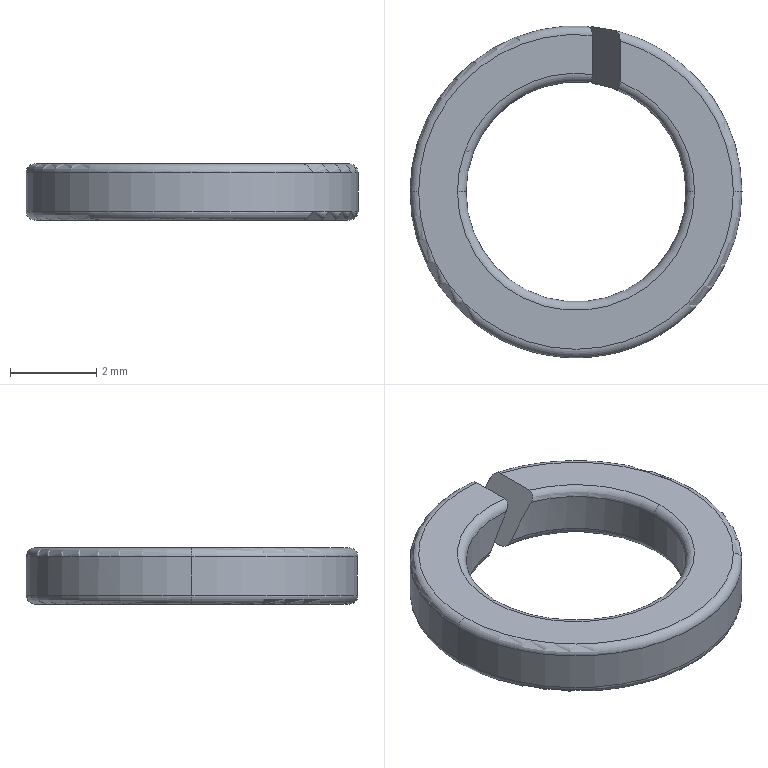Part | STEP file | 弹垫-5^EDA50-R04 (D60N) | 1 solid | 22 faces | box 7.7 x 7.7 x 1.3 mm | volume 32.202 mm3 | torus 12 | cylinder 6 | plane 4 | commonest cylinder face diameters 5.1 x3 7.7 x3